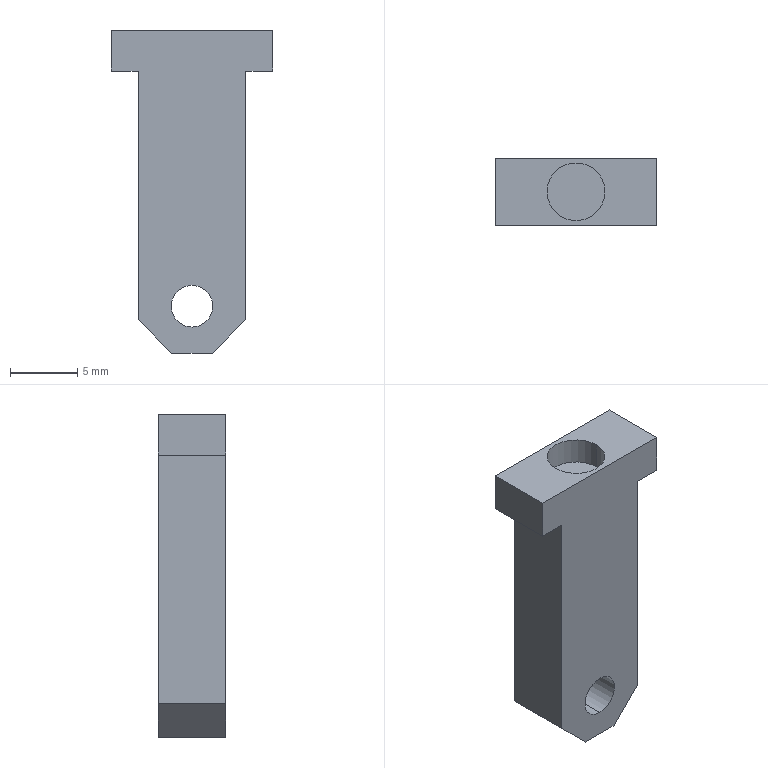Part | NX | features BREP 1 | 1 solid | 17 faces | box 12 x 5 x 24 mm | volume 921.968 mm3 | plane 13 | cylinder 4 | commonest cylinder face diameters 3.1 x2 4.3 x2
STEP:
#1=CARTESIAN_POINT('',(-2.15,0.,-2.));
#2=VERTEX_POINT('',#1);
#3=CARTESIAN_POINT('',(2.15,0.,-2.));
#4=VERTEX_POINT('',#3);
#5=CARTESIAN_POINT('',(0.,0.,-2.));
#6=DIRECTION('',(0.,0.,1.));
#7=DIRECTION('',(1.,0.,0.));
#8=AXIS2_PLACEMENT_3D('',#5,#6,#7);
#9=CIRCLE('',#8,2.15);
#10=EDGE_CURVE('',#2,#4,#9,.T.);
#11=ORIENTED_EDGE('',*,*,#10,.F.);
#12=CARTESIAN_POINT('',(-2.15,0.,0.));
#13=VERTEX_POINT('',#12);
#14=CARTESIAN_POINT('',(-2.15,0.,-2.));
#15=DIRECTION('',(0.,0.,1.));
#16=VECTOR('',#15,1000.);
#17=LINE('',#14,#16);
#18=EDGE_CURVE('',#2,#13,#17,.T.);
#19=ORIENTED_EDGE('',*,*,#18,.T.);
#20=CARTESIAN_POINT('',(2.15,0.,0.));
#21=VERTEX_POINT('',#20);
#22=CARTESIAN_POINT('',(0.,0.,0.));
#23=DIRECTION('',(0.,0.,1.));
#24=DIRECTION('',(1.,0.,0.));
#25=AXIS2_PLACEMENT_3D('',#22,#23,#24);
#26=CIRCLE('',#25,2.15);
#27=EDGE_CURVE('',#13,#21,#26,.T.);
#28=ORIENTED_EDGE('',*,*,#27,.T.);
#29=CARTESIAN_POINT('',(2.15,0.,-2.));
#30=DIRECTION('',(0.,0.,1.));
#31=VECTOR('',#30,1000.);
#32=LINE('',#29,#31);
#33=EDGE_CURVE('',#4,#21,#32,.T.);
#34=ORIENTED_EDGE('',*,*,#33,.F.);
#35=EDGE_LOOP('',(#11,#19,#28,#34));
#36=FACE_BOUND('',#35,.T.);
#37=CARTESIAN_POINT('',(0.,0.,-2.));
#38=DIRECTION('',(0.,0.,1.));
#39=DIRECTION('',(-1.,0.,0.));
#40=AXIS2_PLACEMENT_3D('',#37,#38,#39);
#41=CYLINDRICAL_SURFACE('',#40,2.15);
#42=ADVANCED_FACE('',(#36),#41,.F.);
#43=CARTESIAN_POINT('',(0.,-2.5,-22.05));
#44=VERTEX_POINT('',#43);
#45=CARTESIAN_POINT('',(0.,-2.5,-18.95));
#46=VERTEX_POINT('',#45);
#47=CARTESIAN_POINT('',(0.,-2.5,-20.5));
#48=DIRECTION('',(0.,1.,0.));
#49=DIRECTION('',(0.,0.,1.));
#50=AXIS2_PLACEMENT_3D('',#47,#48,#49);
#51=CIRCLE('',#50,1.55);
#52=EDGE_CURVE('',#44,#46,#51,.T.);
#53=ORIENTED_EDGE('',*,*,#52,.F.);
#54=CARTESIAN_POINT('',(0.,2.5,-22.05));
#55=VERTEX_POINT('',#54);
#56=CARTESIAN_POINT('',(0.,-2.5,-22.05));
#57=DIRECTION('',(0.,1.,0.));
#58=VECTOR('',#57,1000.);
#59=LINE('',#56,#58);
#60=EDGE_CURVE('',#44,#55,#59,.T.);
#61=ORIENTED_EDGE('',*,*,#60,.T.);
#62=CARTESIAN_POINT('',(0.,2.5,-18.95));
#63=VERTEX_POINT('',#62);
#64=CARTESIAN_POINT('',(0.,2.5,-20.5));
#65=DIRECTION('',(0.,1.,0.));
#66=DIRECTION('',(0.,0.,1.));
#67=AXIS2_PLACEMENT_3D('',#64,#65,#66);
#68=CIRCLE('',#67,1.55);
#69=EDGE_CURVE('',#55,#63,#68,.T.);
#70=ORIENTED_EDGE('',*,*,#69,.T.);
#71=CARTESIAN_POINT('',(0.,-2.5,-18.95));
#72=DIRECTION('',(0.,1.,0.));
#73=VECTOR('',#72,1000.);
#74=LINE('',#71,#73);
#75=EDGE_CURVE('',#46,#63,#74,.T.);
#76=ORIENTED_EDGE('',*,*,#75,.F.);
#77=EDGE_LOOP('',(#53,#61,#70,#76));
#78=FACE_BOUND('',#77,.T.);
#79=CARTESIAN_POINT('',(0.,-2.5,-20.5));
#80=DIRECTION('',(0.,1.,0.));
#81=DIRECTION('',(0.,0.,-1.));
#82=AXIS2_PLACEMENT_3D('',#79,#80,#81);
#83=CYLINDRICAL_SURFACE('',#82,1.55);
#84=ADVANCED_FACE('',(#78),#83,.F.);
#85=CARTESIAN_POINT('',(4.,-2.5,-3.));
#86=VERTEX_POINT('',#85);
#87=CARTESIAN_POINT('',(4.,-2.5,-21.5));
#88=VERTEX_POINT('',#87);
#89=CARTESIAN_POINT('',(4.,-2.5,-24.));
#90=DIRECTION('',(0.,0.,-1.));
#91=VECTOR('',#90,1000.);
#92=LINE('',#89,#91);
#93=EDGE_CURVE('',#86,#88,#92,.T.);
#94=ORIENTED_EDGE('',*,*,#93,.T.);
#95=CARTESIAN_POINT('',(4.,2.5,-21.5));
#96=VERTEX_POINT('',#95);
#97=CARTESIAN_POINT('',(4.,2.5,-21.5));
#98=DIRECTION('',(0.,1.,0.));
#99=VECTOR('',#98,1000.);
#100=LINE('',#97,#99);
#101=EDGE_CURVE('',#88,#96,#100,.T.);
#102=ORIENTED_EDGE('',*,*,#101,.T.);
#103=CARTESIAN_POINT('',(4.,2.5,-3.));
#104=VERTEX_POINT('',#103);
#105=CARTESIAN_POINT('',(4.,2.5,-24.));
#106=DIRECTION('',(0.,0.,-1.));
#107=VECTOR('',#106,1000.);
#108=LINE('',#105,#107);
#109=EDGE_CURVE('',#104,#96,#108,.T.);
#110=ORIENTED_EDGE('',*,*,#109,.F.);
#111=CARTESIAN_POINT('',(4.,2.5,-3.));
#112=DIRECTION('',(0.,-1.,0.));
#113=VECTOR('',#112,1000.);
#114=LINE('',#111,#113);
#115=EDGE_CURVE('',#104,#86,#114,.T.);
#116=ORIENTED_EDGE('',*,*,#115,.T.);
#117=EDGE_LOOP('',(#94,#102,#110,#116));
#118=FACE_BOUND('',#117,.T.);
#119=CARTESIAN_POINT('',(4.,2.5,-24.));
#120=DIRECTION('',(-1.,0.,0.));
#121=DIRECTION('',(0.,0.,-1.));
#122=AXIS2_PLACEMENT_3D('',#119,#120,#121);
#123=PLANE('',#122);
#124=ADVANCED_FACE('',(#118),#123,.F.);
#125=CARTESIAN_POINT('',(1.5,2.5,-24.));
#126=VERTEX_POINT('',#125);
#127=CARTESIAN_POINT('',(-1.5,2.5,-24.));
#128=VERTEX_POINT('',#127);
#129=CARTESIAN_POINT('',(-4.,2.5,-24.));
#130=DIRECTION('',(-1.,0.,0.));
#131=VECTOR('',#130,1000.);
#132=LINE('',#129,#131);
#133=EDGE_CURVE('',#126,#128,#132,.T.);
#134=ORIENTED_EDGE('',*,*,#133,.F.);
#135=CARTESIAN_POINT('',(1.5,-2.5,-24.));
#136=VERTEX_POINT('',#135);
#137=CARTESIAN_POINT('',(1.5,2.5,-24.));
#138=DIRECTION('',(0.,-1.,0.));
#139=VECTOR('',#138,1000.);
#140=LINE('',#137,#139);
#141=EDGE_CURVE('',#126,#136,#140,.T.);
#142=ORIENTED_EDGE('',*,*,#141,.T.);
#143=CARTESIAN_POINT('',(-1.5,-2.5,-24.));
#144=VERTEX_POINT('',#143);
#145=CARTESIAN_POINT('',(-4.,-2.5,-24.));
#146=DIRECTION('',(-1.,0.,0.));
#147=VECTOR('',#146,1000.);
#148=LINE('',#145,#147);
#149=EDGE_CURVE('',#136,#144,#148,.T.);
#150=ORIENTED_EDGE('',*,*,#149,.T.);
#151=CARTESIAN_POINT('',(-1.5,2.5,-24.));
#152=DIRECTION('',(0.,1.,0.));
#153=VECTOR('',#152,1000.);
#154=LINE('',#151,#153);
#155=EDGE_CURVE('',#144,#128,#154,.T.);
#156=ORIENTED_EDGE('',*,*,#155,.T.);
#157=EDGE_LOOP('',(#134,#142,#150,#156));
#158=FACE_BOUND('',#157,.T.);
#159=CARTESIAN_POINT('',(-4.,2.5,-24.));
#160=DIRECTION('',(0.,0.,1.));
#161=DIRECTION('',(-1.,0.,0.));
#162=AXIS2_PLACEMENT_3D('',#159,#160,#161);
#163=PLANE('',#162);
#164=ADVANCED_FACE('',(#158),#163,.F.);
#165=CARTESIAN_POINT('',(-4.,2.5,-21.5));
#166=VERTEX_POINT('',#165);
#167=CARTESIAN_POINT('',(-4.,2.5,-3.));
#168=VERTEX_POINT('',#167);
#169=CARTESIAN_POINT('',(-4.,2.5,-24.));
#170=DIRECTION('',(0.,0.,1.));
#171=VECTOR('',#170,1000.);
#172=LINE('',#169,#171);
#173=EDGE_CURVE('',#166,#168,#172,.T.);
#174=ORIENTED_EDGE('',*,*,#173,.F.);
#175=CARTESIAN_POINT('',(-4.,-2.5,-21.5));
#176=VERTEX_POINT('',#175);
#177=CARTESIAN_POINT('',(-4.,2.5,-21.5));
#178=DIRECTION('',(0.,-1.,0.));
#179=VECTOR('',#178,1000.);
#180=LINE('',#177,#179);
#181=EDGE_CURVE('',#166,#176,#180,.T.);
#182=ORIENTED_EDGE('',*,*,#181,.T.);
#183=CARTESIAN_POINT('',(-4.,-2.5,-3.));
#184=VERTEX_POINT('',#183);
#185=CARTESIAN_POINT('',(-4.,-2.5,-24.));
#186=DIRECTION('',(0.,0.,1.));
#187=VECTOR('',#186,1000.);
#188=LINE('',#185,#187);
#189=EDGE_CURVE('',#176,#184,#188,.T.);
#190=ORIENTED_EDGE('',*,*,#189,.T.);
#191=CARTESIAN_POINT('',(-4.,2.5,-3.));
#192=DIRECTION('',(0.,-1.,0.));
#193=VECTOR('',#192,1000.);
#194=LINE('',#191,#193);
#195=EDGE_CURVE('',#168,#184,#194,.T.);
#196=ORIENTED_EDGE('',*,*,#195,.F.);
#197=EDGE_LOOP('',(#174,#182,#190,#196));
#198=FACE_BOUND('',#197,.T.);
#199=CARTESIAN_POINT('',(-4.,2.5,-24.));
#200=DIRECTION('',(1.,0.,0.));
#201=DIRECTION('',(0.,0.,1.));
#202=AXIS2_PLACEMENT_3D('',#199,#200,#201);
#203=PLANE('',#202);
#204=ADVANCED_FACE('',(#198),#203,.F.);
#205=CARTESIAN_POINT('',(-6.,-2.5,-3.));
#206=VERTEX_POINT('',#205);
#207=CARTESIAN_POINT('',(-4.,-2.5,-3.));
#208=DIRECTION('',(-1.,0.,0.));
#209=VECTOR('',#208,1000.);
#210=LINE('',#207,#209);
#211=EDGE_CURVE('',#184,#206,#210,.T.);
#212=ORIENTED_EDGE('',*,*,#211,.T.);
#213=CARTESIAN_POINT('',(-6.,2.5,-3.));
#214=VERTEX_POINT('',#213);
#215=CARTESIAN_POINT('',(-6.,2.5,-3.));
#216=DIRECTION('',(0.,-1.,0.));
#217=VECTOR('',#216,1000.);
#218=LINE('',#215,#217);
#219=EDGE_CURVE('',#214,#206,#218,.T.);
#220=ORIENTED_EDGE('',*,*,#219,.F.);
#221=CARTESIAN_POINT('',(-4.,2.5,-3.));
#222=DIRECTION('',(-1.,0.,0.));
#223=VECTOR('',#222,1000.);
#224=LINE('',#221,#223);
#225=EDGE_CURVE('',#168,#214,#224,.T.);
#226=ORIENTED_EDGE('',*,*,#225,.F.);
#227=ORIENTED_EDGE('',*,*,#195,.T.);
#228=EDGE_LOOP('',(#212,#220,#226,#227));
#229=FACE_BOUND('',#228,.T.);
#230=CARTESIAN_POINT('',(-4.,2.5,-3.));
#231=DIRECTION('',(0.,0.,1.));
#232=DIRECTION('',(-1.,0.,0.));
#233=AXIS2_PLACEMENT_3D('',#230,#231,#232);
#234=PLANE('',#233);
#235=ADVANCED_FACE('',(#229),#234,.F.);
#236=CARTESIAN_POINT('',(-6.,-2.5,0.));
#237=VERTEX_POINT('',#236);
#238=CARTESIAN_POINT('',(-6.,-2.5,-3.));
#239=DIRECTION('',(0.,0.,1.));
#240=VECTOR('',#239,1000.);
#241=LINE('',#238,#240);
#242=EDGE_CURVE('',#206,#237,#241,.T.);
#243=ORIENTED_EDGE('',*,*,#242,.T.);
#244=CARTESIAN_POINT('',(-6.,2.5,0.));
#245=VERTEX_POINT('',#244);
#246=CARTESIAN_POINT('',(-6.,2.5,0.));
#247=DIRECTION('',(0.,-1.,0.));
#248=VECTOR('',#247,1000.);
#249=LINE('',#246,#248);
#250=EDGE_CURVE('',#245,#237,#249,.T.);
#251=ORIENTED_EDGE('',*,*,#250,.F.);
#252=CARTESIAN_POINT('',(-6.,2.5,-3.));
#253=DIRECTION('',(0.,0.,1.));
#254=VECTOR('',#253,1000.);
#255=LINE('',#252,#254);
#256=EDGE_CURVE('',#214,#245,#255,.T.);
#257=ORIENTED_EDGE('',*,*,#256,.F.);
#258=ORIENTED_EDGE('',*,*,#219,.T.);
#259=EDGE_LOOP('',(#243,#251,#257,#258));
#260=FACE_BOUND('',#259,.T.);
#261=CARTESIAN_POINT('',(-6.,2.5,-3.));
#262=DIRECTION('',(1.,0.,0.));
#263=DIRECTION('',(0.,0.,1.));
#264=AXIS2_PLACEMENT_3D('',#261,#262,#263);
#265=PLANE('',#264);
#266=ADVANCED_FACE('',(#260),#265,.F.);
#267=CARTESIAN_POINT('',(0.,0.,0.));
#268=DIRECTION('',(0.,0.,1.));
#269=DIRECTION('',(1.,0.,0.));
#270=AXIS2_PLACEMENT_3D('',#267,#268,#269);
#271=CIRCLE('',#270,2.15);
#272=EDGE_CURVE('',#21,#13,#271,.T.);
#273=ORIENTED_EDGE('',*,*,#272,.F.);
#274=ORIENTED_EDGE('',*,*,#27,.F.);
#275=EDGE_LOOP('',(#273,#274));
#276=FACE_BOUND('',#275,.T.);
#277=CARTESIAN_POINT('',(6.,-2.5,0.));
#278=VERTEX_POINT('',#277);
#279=CARTESIAN_POINT('',(6.,-2.5,0.));
#280=DIRECTION('',(1.,0.,0.));
#281=VECTOR('',#280,1000.);
#282=LINE('',#279,#281);
#283=EDGE_CURVE('',#237,#278,#282,.T.);
#284=ORIENTED_EDGE('',*,*,#283,.T.);
#285=CARTESIAN_POINT('',(6.,2.5,0.));
#286=VERTEX_POINT('',#285);
#287=CARTESIAN_POINT('',(6.,2.5,0.));
#288=DIRECTION('',(0.,-1.,0.));
#289=VECTOR('',#288,1000.);
#290=LINE('',#287,#289);
#291=EDGE_CURVE('',#286,#278,#290,.T.);
#292=ORIENTED_EDGE('',*,*,#291,.F.);
#293=CARTESIAN_POINT('',(6.,2.5,0.));
#294=DIRECTION('',(1.,0.,0.));
#295=VECTOR('',#294,1000.);
#296=LINE('',#293,#295);
#297=EDGE_CURVE('',#245,#286,#296,.T.);
#298=ORIENTED_EDGE('',*,*,#297,.F.);
#299=ORIENTED_EDGE('',*,*,#250,.T.);
#300=EDGE_LOOP('',(#284,#292,#298,#299));
#301=FACE_BOUND('',#300,.T.);
#302=CARTESIAN_POINT('',(6.,2.5,0.));
#303=DIRECTION('',(0.,0.,-1.));
#304=DIRECTION('',(1.,0.,0.));
#305=AXIS2_PLACEMENT_3D('',#302,#303,#304);
#306=PLANE('',#305);
#307=ADVANCED_FACE('',(#276,#301),#306,.F.);
#308=CARTESIAN_POINT('',(6.,-2.5,-3.));
#309=VERTEX_POINT('',#308);
#310=CARTESIAN_POINT('',(6.,-2.5,-3.));
#311=DIRECTION('',(0.,0.,-1.));
#312=VECTOR('',#311,1000.);
#313=LINE('',#310,#312);
#314=EDGE_CURVE('',#278,#309,#313,.T.);
#315=ORIENTED_EDGE('',*,*,#314,.T.);
#316=CARTESIAN_POINT('',(6.,2.5,-3.));
#317=VERTEX_POINT('',#316);
#318=CARTESIAN_POINT('',(6.,2.5,-3.));
#319=DIRECTION('',(0.,-1.,0.));
#320=VECTOR('',#319,1000.);
#321=LINE('',#318,#320);
#322=EDGE_CURVE('',#317,#309,#321,.T.);
#323=ORIENTED_EDGE('',*,*,#322,.F.);
#324=CARTESIAN_POINT('',(6.,2.5,-3.));
#325=DIRECTION('',(0.,0.,-1.));
#326=VECTOR('',#325,1000.);
#327=LINE('',#324,#326);
#328=EDGE_CURVE('',#286,#317,#327,.T.);
#329=ORIENTED_EDGE('',*,*,#328,.F.);
#330=ORIENTED_EDGE('',*,*,#291,.T.);
#331=EDGE_LOOP('',(#315,#323,#329,#330));
#332=FACE_BOUND('',#331,.T.);
#333=CARTESIAN_POINT('',(6.,2.5,-3.));
#334=DIRECTION('',(-1.,0.,0.));
#335=DIRECTION('',(0.,0.,-1.));
#336=AXIS2_PLACEMENT_3D('',#333,#334,#335);
#337=PLANE('',#336);
#338=ADVANCED_FACE('',(#332),#337,.F.);
#339=CARTESIAN_POINT('',(4.,-2.5,-3.));
#340=DIRECTION('',(-1.,0.,0.));
#341=VECTOR('',#340,1000.);
#342=LINE('',#339,#341);
#343=EDGE_CURVE('',#309,#86,#342,.T.);
#344=ORIENTED_EDGE('',*,*,#343,.T.);
#345=ORIENTED_EDGE('',*,*,#115,.F.);
#346=CARTESIAN_POINT('',(4.,2.5,-3.));
#347=DIRECTION('',(-1.,0.,0.));
#348=VECTOR('',#347,1000.);
#349=LINE('',#346,#348);
#350=EDGE_CURVE('',#317,#104,#349,.T.);
#351=ORIENTED_EDGE('',*,*,#350,.F.);
#352=ORIENTED_EDGE('',*,*,#322,.T.);
#353=EDGE_LOOP('',(#344,#345,#351,#352));
#354=FACE_BOUND('',#353,.T.);
#355=CARTESIAN_POINT('',(4.,2.5,-3.));
#356=DIRECTION('',(0.,0.,1.));
#357=DIRECTION('',(-1.,0.,0.));
#358=AXIS2_PLACEMENT_3D('',#355,#356,#357);
#359=PLANE('',#358);
#360=ADVANCED_FACE('',(#354),#359,.F.);
#361=CARTESIAN_POINT('',(0.,2.5,-20.5));
#362=DIRECTION('',(0.,1.,0.));
#363=DIRECTION('',(0.,0.,1.));
#364=AXIS2_PLACEMENT_3D('',#361,#362,#363);
#365=CIRCLE('',#364,1.55);
#366=EDGE_CURVE('',#63,#55,#365,.T.);
#367=ORIENTED_EDGE('',*,*,#366,.F.);
#368=ORIENTED_EDGE('',*,*,#69,.F.);
#369=EDGE_LOOP('',(#367,#368));
#370=FACE_BOUND('',#369,.T.);
#371=ORIENTED_EDGE('',*,*,#109,.T.);
#372=CARTESIAN_POINT('',(12.75,2.5,-12.75));
#373=DIRECTION('',(-0.7071,0.,-0.7071));
#374=VECTOR('',#373,1000.);
#375=LINE('',#372,#374);
#376=EDGE_CURVE('',#96,#126,#375,.T.);
#377=ORIENTED_EDGE('',*,*,#376,.T.);
#378=ORIENTED_EDGE('',*,*,#133,.T.);
#379=CARTESIAN_POINT('',(-12.75,2.5,-12.75));
#380=DIRECTION('',(-0.7071,0.,0.7071));
#381=VECTOR('',#380,1000.);
#382=LINE('',#379,#381);
#383=EDGE_CURVE('',#128,#166,#382,.T.);
#384=ORIENTED_EDGE('',*,*,#383,.T.);
#385=ORIENTED_EDGE('',*,*,#173,.T.);
#386=ORIENTED_EDGE('',*,*,#225,.T.);
#387=ORIENTED_EDGE('',*,*,#256,.T.);
#388=ORIENTED_EDGE('',*,*,#297,.T.);
#389=ORIENTED_EDGE('',*,*,#328,.T.);
#390=ORIENTED_EDGE('',*,*,#350,.T.);
#391=EDGE_LOOP('',(#371,#377,#378,#384,#385,#386,#387,#388,#389,#390));
#392=FACE_BOUND('',#391,.T.);
#393=CARTESIAN_POINT('',(0.,2.5,0.));
#394=DIRECTION('',(0.,1.,0.));
#395=DIRECTION('',(0.,0.,-1.));
#396=AXIS2_PLACEMENT_3D('',#393,#394,#395);
#397=PLANE('',#396);
#398=ADVANCED_FACE('',(#370,#392),#397,.T.);
#399=CARTESIAN_POINT('',(0.,-2.5,-20.5));
#400=DIRECTION('',(0.,1.,0.));
#401=DIRECTION('',(0.,0.,1.));
#402=AXIS2_PLACEMENT_3D('',#399,#400,#401);
#403=CIRCLE('',#402,1.55);
#404=EDGE_CURVE('',#46,#44,#403,.T.);
#405=ORIENTED_EDGE('',*,*,#404,.T.);
#406=ORIENTED_EDGE('',*,*,#52,.T.);
#407=EDGE_LOOP('',(#405,#406));
#408=FACE_BOUND('',#407,.T.);
#409=ORIENTED_EDGE('',*,*,#149,.F.);
#410=CARTESIAN_POINT('',(1.5,-2.5,-24.));
#411=DIRECTION('',(0.7071,0.,0.7071));
#412=VECTOR('',#411,1000.);
#413=LINE('',#410,#412);
#414=EDGE_CURVE('',#136,#88,#413,.T.);
#415=ORIENTED_EDGE('',*,*,#414,.T.);
#416=ORIENTED_EDGE('',*,*,#93,.F.);
#417=ORIENTED_EDGE('',*,*,#343,.F.);
#418=ORIENTED_EDGE('',*,*,#314,.F.);
#419=ORIENTED_EDGE('',*,*,#283,.F.);
#420=ORIENTED_EDGE('',*,*,#242,.F.);
#421=ORIENTED_EDGE('',*,*,#211,.F.);
#422=ORIENTED_EDGE('',*,*,#189,.F.);
#423=CARTESIAN_POINT('',(-4.,-2.5,-21.5));
#424=DIRECTION('',(0.7071,0.,-0.7071));
#425=VECTOR('',#424,1000.);
#426=LINE('',#423,#425);
#427=EDGE_CURVE('',#176,#144,#426,.T.);
#428=ORIENTED_EDGE('',*,*,#427,.T.);
#429=EDGE_LOOP('',(#409,#415,#416,#417,#418,#419,#420,#421,#422,#428));
#430=FACE_BOUND('',#429,.T.);
#431=CARTESIAN_POINT('',(0.,-2.5,0.));
#432=DIRECTION('',(0.,1.,0.));
#433=DIRECTION('',(0.,0.,-1.));
#434=AXIS2_PLACEMENT_3D('',#431,#432,#433);
#435=PLANE('',#434);
#436=ADVANCED_FACE('',(#408,#430),#435,.F.);
#437=ORIENTED_EDGE('',*,*,#60,.F.);
#438=ORIENTED_EDGE('',*,*,#404,.F.);
#439=ORIENTED_EDGE('',*,*,#75,.T.);
#440=ORIENTED_EDGE('',*,*,#366,.T.);
#441=EDGE_LOOP('',(#437,#438,#439,#440));
#442=FACE_BOUND('',#441,.T.);
#443=CARTESIAN_POINT('',(0.,-2.5,-20.5));
#444=DIRECTION('',(0.,1.,0.));
#445=DIRECTION('',(0.,0.,-1.));
#446=AXIS2_PLACEMENT_3D('',#443,#444,#445);
#447=CYLINDRICAL_SURFACE('',#446,1.55);
#448=ADVANCED_FACE('',(#442),#447,.F.);
#449=ORIENTED_EDGE('',*,*,#376,.F.);
#450=ORIENTED_EDGE('',*,*,#101,.F.);
#451=ORIENTED_EDGE('',*,*,#414,.F.);
#452=ORIENTED_EDGE('',*,*,#141,.F.);
#453=EDGE_LOOP('',(#449,#450,#451,#452));
#454=FACE_BOUND('',#453,.T.);
#455=CARTESIAN_POINT('',(1.5,2.5,-24.));
#456=DIRECTION('',(-0.7071,0.,0.7071));
#457=DIRECTION('',(0.,1.,0.));
#458=AXIS2_PLACEMENT_3D('',#455,#456,#457);
#459=PLANE('',#458);
#460=ADVANCED_FACE('',(#454),#459,.F.);
#461=ORIENTED_EDGE('',*,*,#383,.F.);
#462=ORIENTED_EDGE('',*,*,#155,.F.);
#463=ORIENTED_EDGE('',*,*,#427,.F.);
#464=ORIENTED_EDGE('',*,*,#181,.F.);
#465=EDGE_LOOP('',(#461,#462,#463,#464));
#466=FACE_BOUND('',#465,.T.);
#467=CARTESIAN_POINT('',(-4.,2.5,-21.5));
#468=DIRECTION('',(0.7071,0.,0.7071));
#469=DIRECTION('',(0.,1.,0.));
#470=AXIS2_PLACEMENT_3D('',#467,#468,#469);
#471=PLANE('',#470);
#472=ADVANCED_FACE('',(#466),#471,.F.);
#473=ORIENTED_EDGE('',*,*,#18,.F.);
#474=CARTESIAN_POINT('',(0.,0.,-2.));
#475=DIRECTION('',(0.,0.,1.));
#476=DIRECTION('',(1.,0.,0.));
#477=AXIS2_PLACEMENT_3D('',#474,#475,#476);
#478=CIRCLE('',#477,2.15);
#479=EDGE_CURVE('',#4,#2,#478,.T.);
#480=ORIENTED_EDGE('',*,*,#479,.F.);
#481=ORIENTED_EDGE('',*,*,#33,.T.);
#482=ORIENTED_EDGE('',*,*,#272,.T.);
#483=EDGE_LOOP('',(#473,#480,#481,#482));
#484=FACE_BOUND('',#483,.T.);
#485=CARTESIAN_POINT('',(0.,0.,-2.));
#486=DIRECTION('',(0.,0.,1.));
#487=DIRECTION('',(-1.,0.,0.));
#488=AXIS2_PLACEMENT_3D('',#485,#486,#487);
#489=CYLINDRICAL_SURFACE('',#488,2.15);
#490=ADVANCED_FACE('',(#484),#489,.F.);
#491=ORIENTED_EDGE('',*,*,#479,.T.);
#492=ORIENTED_EDGE('',*,*,#10,.T.);
#493=EDGE_LOOP('',(#491,#492));
#494=FACE_BOUND('',#493,.T.);
#495=CARTESIAN_POINT('',(0.,0.,-2.));
#496=DIRECTION('',(0.,0.,1.));
#497=DIRECTION('',(-1.,0.,0.));
#498=AXIS2_PLACEMENT_3D('',#495,#496,#497);
#499=PLANE('',#498);
#500=ADVANCED_FACE('',(#494),#499,.T.);
#501=CLOSED_SHELL('',(#42,#84,#124,#164,#204,#235,#266,#307,#338,#360,#398,#436,#448,#460,#472,#490,#500));
#502=MANIFOLD_SOLID_BREP('',#501);
#503=(LENGTH_UNIT()NAMED_UNIT(*)SI_UNIT(.MILLI.,.METRE.));
#504=UNCERTAINTY_MEASURE_WITH_UNIT(LENGTH_MEASURE(0.00001),#503,'','');
#505=(NAMED_UNIT(*)PLANE_ANGLE_UNIT()SI_UNIT($,.RADIAN.));
#506=(NAMED_UNIT(*)SI_UNIT($,.STERADIAN.)SOLID_ANGLE_UNIT());
#507=(GEOMETRIC_REPRESENTATION_CONTEXT(3)GLOBAL_UNCERTAINTY_ASSIGNED_CONTEXT((#504))GLOBAL_UNIT_ASSIGNED_CONTEXT((#503,#505,#506))REPRESENTATION_CONTEXT('',''));
#508=ADVANCED_BREP_SHAPE_REPRESENTATION('',(#502),#507);